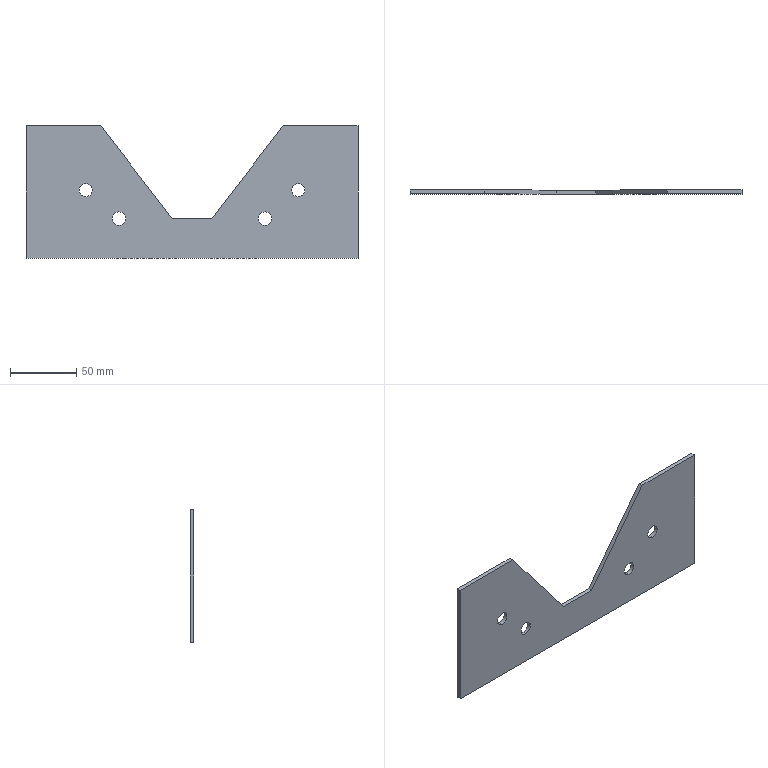Part | SolidWorks | features BaseBody 1 | 1 solid | 18 faces | box 250 x 3 x 100 mm | volume 56478 mm3 | plane 10 | cylinder 8 | commonest cylinder face diameters 10 x8
STEP:
#1=CARTESIAN_POINT('',(437.247,540.,-287.909));
#2=VERTEX_POINT('',#1);
#3=CARTESIAN_POINT('',(437.247,540.,-297.909));
#4=VERTEX_POINT('',#3);
#5=CARTESIAN_POINT('',(437.247,540.,-292.909));
#6=DIRECTION('',(0.,-1.,0.));
#7=DIRECTION('',(0.,0.,-1.));
#8=AXIS2_PLACEMENT_3D('',#5,#6,#7);
#9=CIRCLE('',#8,5.);
#10=EDGE_CURVE('',#2,#4,#9,.T.);
#11=ORIENTED_EDGE('',*,*,#10,.F.);
#12=CARTESIAN_POINT('',(437.247,537.,-287.909));
#13=VERTEX_POINT('',#12);
#14=CARTESIAN_POINT('',(437.247,547.,-287.909));
#15=DIRECTION('',(0.,-1.,0.));
#16=VECTOR('',#15,1000.);
#17=LINE('',#14,#16);
#18=EDGE_CURVE('',#2,#13,#17,.T.);
#19=ORIENTED_EDGE('',*,*,#18,.T.);
#20=CARTESIAN_POINT('',(437.247,537.,-297.909));
#21=VERTEX_POINT('',#20);
#22=CARTESIAN_POINT('',(437.247,537.,-292.909));
#23=DIRECTION('',(0.,1.,0.));
#24=DIRECTION('',(0.,0.,-1.));
#25=AXIS2_PLACEMENT_3D('',#22,#23,#24);
#26=CIRCLE('',#25,5.);
#27=EDGE_CURVE('',#21,#13,#26,.T.);
#28=ORIENTED_EDGE('',*,*,#27,.F.);
#29=CARTESIAN_POINT('',(437.247,547.,-297.909));
#30=DIRECTION('',(0.,-1.,0.));
#31=VECTOR('',#30,1000.);
#32=LINE('',#29,#31);
#33=EDGE_CURVE('',#4,#21,#32,.T.);
#34=ORIENTED_EDGE('',*,*,#33,.F.);
#35=EDGE_LOOP('',(#11,#19,#28,#34));
#36=FACE_OUTER_BOUND('',#35,.T.);
#37=CARTESIAN_POINT('',(437.247,547.,-292.909));
#38=DIRECTION('',(0.,-1.,0.));
#39=DIRECTION('',(0.,0.,-1.));
#40=AXIS2_PLACEMENT_3D('',#37,#38,#39);
#41=CYLINDRICAL_SURFACE('',#40,5.);
#42=ADVANCED_FACE('',(#36),#41,.F.);
#43=CARTESIAN_POINT('',(302.247,540.,-309.345));
#44=VERTEX_POINT('',#43);
#45=CARTESIAN_POINT('',(302.247,540.,-319.345));
#46=VERTEX_POINT('',#45);
#47=CARTESIAN_POINT('',(302.247,540.,-314.345));
#48=DIRECTION('',(0.,-1.,0.));
#49=DIRECTION('',(0.,0.,-1.));
#50=AXIS2_PLACEMENT_3D('',#47,#48,#49);
#51=CIRCLE('',#50,5.);
#52=EDGE_CURVE('',#44,#46,#51,.T.);
#53=ORIENTED_EDGE('',*,*,#52,.F.);
#54=CARTESIAN_POINT('',(302.247,537.,-309.345));
#55=VERTEX_POINT('',#54);
#56=CARTESIAN_POINT('',(302.247,547.,-309.345));
#57=DIRECTION('',(0.,-1.,0.));
#58=VECTOR('',#57,1000.);
#59=LINE('',#56,#58);
#60=EDGE_CURVE('',#44,#55,#59,.T.);
#61=ORIENTED_EDGE('',*,*,#60,.T.);
#62=CARTESIAN_POINT('',(302.247,537.,-319.345));
#63=VERTEX_POINT('',#62);
#64=CARTESIAN_POINT('',(302.247,537.,-314.345));
#65=DIRECTION('',(0.,1.,0.));
#66=DIRECTION('',(0.,0.,-1.));
#67=AXIS2_PLACEMENT_3D('',#64,#65,#66);
#68=CIRCLE('',#67,5.);
#69=EDGE_CURVE('',#63,#55,#68,.T.);
#70=ORIENTED_EDGE('',*,*,#69,.F.);
#71=CARTESIAN_POINT('',(302.247,547.,-319.345));
#72=DIRECTION('',(0.,-1.,0.));
#73=VECTOR('',#72,1000.);
#74=LINE('',#71,#73);
#75=EDGE_CURVE('',#46,#63,#74,.T.);
#76=ORIENTED_EDGE('',*,*,#75,.F.);
#77=EDGE_LOOP('',(#53,#61,#70,#76));
#78=FACE_OUTER_BOUND('',#77,.T.);
#79=CARTESIAN_POINT('',(302.247,547.,-314.345));
#80=DIRECTION('',(0.,-1.,0.));
#81=DIRECTION('',(0.,0.,-1.));
#82=AXIS2_PLACEMENT_3D('',#79,#80,#81);
#83=CYLINDRICAL_SURFACE('',#82,5.);
#84=ADVANCED_FACE('',(#78),#83,.F.);
#85=CARTESIAN_POINT('',(412.247,540.,-309.345));
#86=VERTEX_POINT('',#85);
#87=CARTESIAN_POINT('',(412.247,540.,-319.345));
#88=VERTEX_POINT('',#87);
#89=CARTESIAN_POINT('',(412.247,540.,-314.345));
#90=DIRECTION('',(0.,-1.,0.));
#91=DIRECTION('',(0.,0.,-1.));
#92=AXIS2_PLACEMENT_3D('',#89,#90,#91);
#93=CIRCLE('',#92,5.);
#94=EDGE_CURVE('',#86,#88,#93,.T.);
#95=ORIENTED_EDGE('',*,*,#94,.F.);
#96=CARTESIAN_POINT('',(412.247,537.,-309.345));
#97=VERTEX_POINT('',#96);
#98=CARTESIAN_POINT('',(412.247,547.,-309.345));
#99=DIRECTION('',(0.,-1.,0.));
#100=VECTOR('',#99,1000.);
#101=LINE('',#98,#100);
#102=EDGE_CURVE('',#86,#97,#101,.T.);
#103=ORIENTED_EDGE('',*,*,#102,.T.);
#104=CARTESIAN_POINT('',(412.247,537.,-319.345));
#105=VERTEX_POINT('',#104);
#106=CARTESIAN_POINT('',(412.247,537.,-314.345));
#107=DIRECTION('',(0.,1.,0.));
#108=DIRECTION('',(0.,0.,-1.));
#109=AXIS2_PLACEMENT_3D('',#106,#107,#108);
#110=CIRCLE('',#109,5.);
#111=EDGE_CURVE('',#105,#97,#110,.T.);
#112=ORIENTED_EDGE('',*,*,#111,.F.);
#113=CARTESIAN_POINT('',(412.247,547.,-319.345));
#114=DIRECTION('',(0.,-1.,0.));
#115=VECTOR('',#114,1000.);
#116=LINE('',#113,#115);
#117=EDGE_CURVE('',#88,#105,#116,.T.);
#118=ORIENTED_EDGE('',*,*,#117,.F.);
#119=EDGE_LOOP('',(#95,#103,#112,#118));
#120=FACE_OUTER_BOUND('',#119,.T.);
#121=CARTESIAN_POINT('',(412.247,547.,-314.345));
#122=DIRECTION('',(0.,-1.,0.));
#123=DIRECTION('',(0.,0.,-1.));
#124=AXIS2_PLACEMENT_3D('',#121,#122,#123);
#125=CYLINDRICAL_SURFACE('',#124,5.);
#126=ADVANCED_FACE('',(#120),#125,.F.);
#127=CARTESIAN_POINT('',(277.247,540.,-287.909));
#128=VERTEX_POINT('',#127);
#129=CARTESIAN_POINT('',(277.247,540.,-297.909));
#130=VERTEX_POINT('',#129);
#131=CARTESIAN_POINT('',(277.247,540.,-292.909));
#132=DIRECTION('',(0.,-1.,0.));
#133=DIRECTION('',(0.,0.,-1.));
#134=AXIS2_PLACEMENT_3D('',#131,#132,#133);
#135=CIRCLE('',#134,5.);
#136=EDGE_CURVE('',#128,#130,#135,.T.);
#137=ORIENTED_EDGE('',*,*,#136,.F.);
#138=CARTESIAN_POINT('',(277.247,537.,-287.909));
#139=VERTEX_POINT('',#138);
#140=CARTESIAN_POINT('',(277.247,547.,-287.909));
#141=DIRECTION('',(0.,-1.,0.));
#142=VECTOR('',#141,1000.);
#143=LINE('',#140,#142);
#144=EDGE_CURVE('',#128,#139,#143,.T.);
#145=ORIENTED_EDGE('',*,*,#144,.T.);
#146=CARTESIAN_POINT('',(277.247,537.,-297.909));
#147=VERTEX_POINT('',#146);
#148=CARTESIAN_POINT('',(277.247,537.,-292.909));
#149=DIRECTION('',(0.,1.,0.));
#150=DIRECTION('',(0.,0.,-1.));
#151=AXIS2_PLACEMENT_3D('',#148,#149,#150);
#152=CIRCLE('',#151,5.);
#153=EDGE_CURVE('',#147,#139,#152,.T.);
#154=ORIENTED_EDGE('',*,*,#153,.F.);
#155=CARTESIAN_POINT('',(277.247,547.,-297.909));
#156=DIRECTION('',(0.,-1.,0.));
#157=VECTOR('',#156,1000.);
#158=LINE('',#155,#157);
#159=EDGE_CURVE('',#130,#147,#158,.T.);
#160=ORIENTED_EDGE('',*,*,#159,.F.);
#161=EDGE_LOOP('',(#137,#145,#154,#160));
#162=FACE_OUTER_BOUND('',#161,.T.);
#163=CARTESIAN_POINT('',(277.247,547.,-292.909));
#164=DIRECTION('',(0.,-1.,0.));
#165=DIRECTION('',(0.,0.,-1.));
#166=AXIS2_PLACEMENT_3D('',#163,#164,#165);
#167=CYLINDRICAL_SURFACE('',#166,5.);
#168=ADVANCED_FACE('',(#162),#167,.F.);
#169=ORIENTED_EDGE('',*,*,#27,.T.);
#170=CARTESIAN_POINT('',(437.247,537.,-292.909));
#171=DIRECTION('',(0.,1.,0.));
#172=DIRECTION('',(0.,0.,-1.));
#173=AXIS2_PLACEMENT_3D('',#170,#171,#172);
#174=CIRCLE('',#173,5.);
#175=EDGE_CURVE('',#13,#21,#174,.T.);
#176=ORIENTED_EDGE('',*,*,#175,.T.);
#177=EDGE_LOOP('',(#169,#176));
#178=FACE_BOUND('',#177,.T.);
#179=ORIENTED_EDGE('',*,*,#69,.T.);
#180=CARTESIAN_POINT('',(302.247,537.,-314.345));
#181=DIRECTION('',(0.,1.,0.));
#182=DIRECTION('',(0.,0.,-1.));
#183=AXIS2_PLACEMENT_3D('',#180,#181,#182);
#184=CIRCLE('',#183,5.);
#185=EDGE_CURVE('',#55,#63,#184,.T.);
#186=ORIENTED_EDGE('',*,*,#185,.T.);
#187=EDGE_LOOP('',(#179,#186));
#188=FACE_BOUND('',#187,.T.);
#189=ORIENTED_EDGE('',*,*,#111,.T.);
#190=CARTESIAN_POINT('',(412.247,537.,-314.345));
#191=DIRECTION('',(0.,1.,0.));
#192=DIRECTION('',(0.,0.,-1.));
#193=AXIS2_PLACEMENT_3D('',#190,#191,#192);
#194=CIRCLE('',#193,5.);
#195=EDGE_CURVE('',#97,#105,#194,.T.);
#196=ORIENTED_EDGE('',*,*,#195,.T.);
#197=EDGE_LOOP('',(#189,#196));
#198=FACE_BOUND('',#197,.T.);
#199=ORIENTED_EDGE('',*,*,#153,.T.);
#200=CARTESIAN_POINT('',(277.247,537.,-292.909));
#201=DIRECTION('',(0.,1.,0.));
#202=DIRECTION('',(0.,0.,-1.));
#203=AXIS2_PLACEMENT_3D('',#200,#201,#202);
#204=CIRCLE('',#203,5.);
#205=EDGE_CURVE('',#139,#147,#204,.T.);
#206=ORIENTED_EDGE('',*,*,#205,.T.);
#207=EDGE_LOOP('',(#199,#206));
#208=FACE_BOUND('',#207,.T.);
#209=CARTESIAN_POINT('',(232.247,537.,-344.345));
#210=VERTEX_POINT('',#209);
#211=CARTESIAN_POINT('',(482.247,537.,-344.345));
#212=VERTEX_POINT('',#211);
#213=CARTESIAN_POINT('',(357.247,537.,-344.345));
#214=DIRECTION('',(1.,0.,0.));
#215=VECTOR('',#214,1000.);
#216=LINE('',#213,#215);
#217=EDGE_CURVE('',#210,#212,#216,.T.);
#218=ORIENTED_EDGE('',*,*,#217,.T.);
#219=CARTESIAN_POINT('',(482.247,537.,-244.345));
#220=VERTEX_POINT('',#219);
#221=CARTESIAN_POINT('',(482.247,537.,-344.345));
#222=DIRECTION('',(0.,0.,1.));
#223=VECTOR('',#222,1000.);
#224=LINE('',#221,#223);
#225=EDGE_CURVE('',#212,#220,#224,.T.);
#226=ORIENTED_EDGE('',*,*,#225,.T.);
#227=CARTESIAN_POINT('',(425.959,537.,-244.345));
#228=VERTEX_POINT('',#227);
#229=CARTESIAN_POINT('',(357.247,537.,-244.345));
#230=DIRECTION('',(-1.,0.,0.));
#231=VECTOR('',#230,1000.);
#232=LINE('',#229,#231);
#233=EDGE_CURVE('',#220,#228,#232,.T.);
#234=ORIENTED_EDGE('',*,*,#233,.T.);
#235=CARTESIAN_POINT('',(372.247,537.,-314.345));
#236=VERTEX_POINT('',#235);
#237=CARTESIAN_POINT('',(425.959,537.,-244.345));
#238=DIRECTION('',(-0.6088,0.,-0.7934));
#239=VECTOR('',#238,1000.);
#240=LINE('',#237,#239);
#241=EDGE_CURVE('',#228,#236,#240,.T.);
#242=ORIENTED_EDGE('',*,*,#241,.T.);
#243=CARTESIAN_POINT('',(342.247,537.,-314.345));
#244=VERTEX_POINT('',#243);
#245=CARTESIAN_POINT('',(357.247,537.,-314.345));
#246=DIRECTION('',(-1.,0.,0.));
#247=VECTOR('',#246,1000.);
#248=LINE('',#245,#247);
#249=EDGE_CURVE('',#236,#244,#248,.T.);
#250=ORIENTED_EDGE('',*,*,#249,.T.);
#251=CARTESIAN_POINT('',(288.534,537.,-244.345));
#252=VERTEX_POINT('',#251);
#253=CARTESIAN_POINT('',(342.247,537.,-314.345));
#254=DIRECTION('',(-0.6088,0.,0.7934));
#255=VECTOR('',#254,1000.);
#256=LINE('',#253,#255);
#257=EDGE_CURVE('',#244,#252,#256,.T.);
#258=ORIENTED_EDGE('',*,*,#257,.T.);
#259=CARTESIAN_POINT('',(232.247,537.,-244.345));
#260=VERTEX_POINT('',#259);
#261=CARTESIAN_POINT('',(357.247,537.,-244.345));
#262=DIRECTION('',(-1.,0.,0.));
#263=VECTOR('',#262,1000.);
#264=LINE('',#261,#263);
#265=EDGE_CURVE('',#252,#260,#264,.T.);
#266=ORIENTED_EDGE('',*,*,#265,.T.);
#267=CARTESIAN_POINT('',(232.247,537.,-344.345));
#268=DIRECTION('',(0.,0.,-1.));
#269=VECTOR('',#268,1000.);
#270=LINE('',#267,#269);
#271=EDGE_CURVE('',#260,#210,#270,.T.);
#272=ORIENTED_EDGE('',*,*,#271,.T.);
#273=EDGE_LOOP('',(#218,#226,#234,#242,#250,#258,#266,#272));
#274=FACE_OUTER_BOUND('',#273,.T.);
#275=CARTESIAN_POINT('',(357.247,537.,-344.345));
#276=DIRECTION('',(0.,-1.,0.));
#277=DIRECTION('',(0.,0.,-1.));
#278=AXIS2_PLACEMENT_3D('',#275,#276,#277);
#279=PLANE('',#278);
#280=ADVANCED_FACE('',(#178,#188,#198,#208,#274),#279,.T.);
#281=ORIENTED_EDGE('',*,*,#18,.F.);
#282=CARTESIAN_POINT('',(437.247,540.,-292.909));
#283=DIRECTION('',(0.,-1.,0.));
#284=DIRECTION('',(0.,0.,-1.));
#285=AXIS2_PLACEMENT_3D('',#282,#283,#284);
#286=CIRCLE('',#285,5.);
#287=EDGE_CURVE('',#4,#2,#286,.T.);
#288=ORIENTED_EDGE('',*,*,#287,.F.);
#289=ORIENTED_EDGE('',*,*,#33,.T.);
#290=ORIENTED_EDGE('',*,*,#175,.F.);
#291=EDGE_LOOP('',(#281,#288,#289,#290));
#292=FACE_OUTER_BOUND('',#291,.T.);
#293=CARTESIAN_POINT('',(437.247,547.,-292.909));
#294=DIRECTION('',(0.,-1.,0.));
#295=DIRECTION('',(0.,0.,-1.));
#296=AXIS2_PLACEMENT_3D('',#293,#294,#295);
#297=CYLINDRICAL_SURFACE('',#296,5.);
#298=ADVANCED_FACE('',(#292),#297,.F.);
#299=ORIENTED_EDGE('',*,*,#60,.F.);
#300=CARTESIAN_POINT('',(302.247,540.,-314.345));
#301=DIRECTION('',(0.,-1.,0.));
#302=DIRECTION('',(0.,0.,-1.));
#303=AXIS2_PLACEMENT_3D('',#300,#301,#302);
#304=CIRCLE('',#303,5.);
#305=EDGE_CURVE('',#46,#44,#304,.T.);
#306=ORIENTED_EDGE('',*,*,#305,.F.);
#307=ORIENTED_EDGE('',*,*,#75,.T.);
#308=ORIENTED_EDGE('',*,*,#185,.F.);
#309=EDGE_LOOP('',(#299,#306,#307,#308));
#310=FACE_OUTER_BOUND('',#309,.T.);
#311=CARTESIAN_POINT('',(302.247,547.,-314.345));
#312=DIRECTION('',(0.,-1.,0.));
#313=DIRECTION('',(0.,0.,-1.));
#314=AXIS2_PLACEMENT_3D('',#311,#312,#313);
#315=CYLINDRICAL_SURFACE('',#314,5.);
#316=ADVANCED_FACE('',(#310),#315,.F.);
#317=ORIENTED_EDGE('',*,*,#102,.F.);
#318=CARTESIAN_POINT('',(412.247,540.,-314.345));
#319=DIRECTION('',(0.,-1.,0.));
#320=DIRECTION('',(0.,0.,-1.));
#321=AXIS2_PLACEMENT_3D('',#318,#319,#320);
#322=CIRCLE('',#321,5.);
#323=EDGE_CURVE('',#88,#86,#322,.T.);
#324=ORIENTED_EDGE('',*,*,#323,.F.);
#325=ORIENTED_EDGE('',*,*,#117,.T.);
#326=ORIENTED_EDGE('',*,*,#195,.F.);
#327=EDGE_LOOP('',(#317,#324,#325,#326));
#328=FACE_OUTER_BOUND('',#327,.T.);
#329=CARTESIAN_POINT('',(412.247,547.,-314.345));
#330=DIRECTION('',(0.,-1.,0.));
#331=DIRECTION('',(0.,0.,-1.));
#332=AXIS2_PLACEMENT_3D('',#329,#330,#331);
#333=CYLINDRICAL_SURFACE('',#332,5.);
#334=ADVANCED_FACE('',(#328),#333,.F.);
#335=ORIENTED_EDGE('',*,*,#144,.F.);
#336=CARTESIAN_POINT('',(277.247,540.,-292.909));
#337=DIRECTION('',(0.,-1.,0.));
#338=DIRECTION('',(0.,0.,-1.));
#339=AXIS2_PLACEMENT_3D('',#336,#337,#338);
#340=CIRCLE('',#339,5.);
#341=EDGE_CURVE('',#130,#128,#340,.T.);
#342=ORIENTED_EDGE('',*,*,#341,.F.);
#343=ORIENTED_EDGE('',*,*,#159,.T.);
#344=ORIENTED_EDGE('',*,*,#205,.F.);
#345=EDGE_LOOP('',(#335,#342,#343,#344));
#346=FACE_OUTER_BOUND('',#345,.T.);
#347=CARTESIAN_POINT('',(277.247,547.,-292.909));
#348=DIRECTION('',(0.,-1.,0.));
#349=DIRECTION('',(0.,0.,-1.));
#350=AXIS2_PLACEMENT_3D('',#347,#348,#349);
#351=CYLINDRICAL_SURFACE('',#350,5.);
#352=ADVANCED_FACE('',(#346),#351,.F.);
#353=ORIENTED_EDGE('',*,*,#225,.F.);
#354=CARTESIAN_POINT('',(482.247,540.,-344.345));
#355=VERTEX_POINT('',#354);
#356=CARTESIAN_POINT('',(482.247,537.,-344.345));
#357=DIRECTION('',(0.,-1.,0.));
#358=VECTOR('',#357,1000.);
#359=LINE('',#356,#358);
#360=EDGE_CURVE('',#355,#212,#359,.T.);
#361=ORIENTED_EDGE('',*,*,#360,.F.);
#362=CARTESIAN_POINT('',(482.247,540.,-244.345));
#363=VERTEX_POINT('',#362);
#364=CARTESIAN_POINT('',(482.247,540.,-344.345));
#365=DIRECTION('',(0.,0.,-1.));
#366=VECTOR('',#365,1000.);
#367=LINE('',#364,#366);
#368=EDGE_CURVE('',#363,#355,#367,.T.);
#369=ORIENTED_EDGE('',*,*,#368,.F.);
#370=CARTESIAN_POINT('',(482.247,537.,-244.345));
#371=DIRECTION('',(0.,1.,0.));
#372=VECTOR('',#371,1000.);
#373=LINE('',#370,#372);
#374=EDGE_CURVE('',#220,#363,#373,.T.);
#375=ORIENTED_EDGE('',*,*,#374,.F.);
#376=EDGE_LOOP('',(#353,#361,#369,#375));
#377=FACE_OUTER_BOUND('',#376,.T.);
#378=CARTESIAN_POINT('',(482.247,537.,-344.345));
#379=DIRECTION('',(-1.,0.,0.));
#380=DIRECTION('',(0.,0.,1.));
#381=AXIS2_PLACEMENT_3D('',#378,#379,#380);
#382=PLANE('',#381);
#383=ADVANCED_FACE('',(#377),#382,.F.);
#384=ORIENTED_EDGE('',*,*,#217,.F.);
#385=CARTESIAN_POINT('',(232.247,540.,-344.345));
#386=VERTEX_POINT('',#385);
#387=CARTESIAN_POINT('',(232.247,537.,-344.345));
#388=DIRECTION('',(0.,-1.,0.));
#389=VECTOR('',#388,1000.);
#390=LINE('',#387,#389);
#391=EDGE_CURVE('',#386,#210,#390,.T.);
#392=ORIENTED_EDGE('',*,*,#391,.F.);
#393=CARTESIAN_POINT('',(232.247,540.,-344.345));
#394=DIRECTION('',(-1.,0.,0.));
#395=VECTOR('',#394,1000.);
#396=LINE('',#393,#395);
#397=EDGE_CURVE('',#355,#386,#396,.T.);
#398=ORIENTED_EDGE('',*,*,#397,.F.);
#399=ORIENTED_EDGE('',*,*,#360,.T.);
#400=EDGE_LOOP('',(#384,#392,#398,#399));
#401=FACE_OUTER_BOUND('',#400,.T.);
#402=CARTESIAN_POINT('',(232.247,537.,-344.345));
#403=DIRECTION('',(0.,0.,1.));
#404=DIRECTION('',(1.,0.,0.));
#405=AXIS2_PLACEMENT_3D('',#402,#403,#404);
#406=PLANE('',#405);
#407=ADVANCED_FACE('',(#401),#406,.F.);
#408=ORIENTED_EDGE('',*,*,#271,.F.);
#409=CARTESIAN_POINT('',(232.247,540.,-244.345));
#410=VERTEX_POINT('',#409);
#411=CARTESIAN_POINT('',(232.247,537.,-244.345));
#412=DIRECTION('',(0.,-1.,0.));
#413=VECTOR('',#412,1000.);
#414=LINE('',#411,#413);
#415=EDGE_CURVE('',#410,#260,#414,.T.);
#416=ORIENTED_EDGE('',*,*,#415,.F.);
#417=CARTESIAN_POINT('',(232.247,540.,-344.345));
#418=DIRECTION('',(0.,0.,1.));
#419=VECTOR('',#418,1000.);
#420=LINE('',#417,#419);
#421=EDGE_CURVE('',#386,#410,#420,.T.);
#422=ORIENTED_EDGE('',*,*,#421,.F.);
#423=ORIENTED_EDGE('',*,*,#391,.T.);
#424=EDGE_LOOP('',(#408,#416,#422,#423));
#425=FACE_OUTER_BOUND('',#424,.T.);
#426=CARTESIAN_POINT('',(232.247,537.,-344.345));
#427=DIRECTION('',(1.,0.,0.));
#428=DIRECTION('',(0.,0.,-1.));
#429=AXIS2_PLACEMENT_3D('',#426,#427,#428);
#430=PLANE('',#429);
#431=ADVANCED_FACE('',(#425),#430,.F.);
#432=ORIENTED_EDGE('',*,*,#265,.F.);
#433=CARTESIAN_POINT('',(288.534,540.,-244.345));
#434=VERTEX_POINT('',#433);
#435=CARTESIAN_POINT('',(288.534,537.,-244.345));
#436=DIRECTION('',(0.,-1.,0.));
#437=VECTOR('',#436,1000.);
#438=LINE('',#435,#437);
#439=EDGE_CURVE('',#434,#252,#438,.T.);
#440=ORIENTED_EDGE('',*,*,#439,.F.);
#441=CARTESIAN_POINT('',(232.247,540.,-244.345));
#442=DIRECTION('',(1.,0.,0.));
#443=VECTOR('',#442,1000.);
#444=LINE('',#441,#443);
#445=EDGE_CURVE('',#410,#434,#444,.T.);
#446=ORIENTED_EDGE('',*,*,#445,.F.);
#447=ORIENTED_EDGE('',*,*,#415,.T.);
#448=EDGE_LOOP('',(#432,#440,#446,#447));
#449=FACE_OUTER_BOUND('',#448,.T.);
#450=CARTESIAN_POINT('',(232.247,537.,-244.345));
#451=DIRECTION('',(0.,0.,-1.));
#452=DIRECTION('',(-1.,0.,0.));
#453=AXIS2_PLACEMENT_3D('',#450,#451,#452);
#454=PLANE('',#453);
#455=ADVANCED_FACE('',(#449),#454,.F.);
#456=ORIENTED_EDGE('',*,*,#257,.F.);
#457=CARTESIAN_POINT('',(342.247,540.,-314.345));
#458=VERTEX_POINT('',#457);
#459=CARTESIAN_POINT('',(342.247,537.,-314.345));
#460=DIRECTION('',(0.,-1.,0.));
#461=VECTOR('',#460,1000.);
#462=LINE('',#459,#461);
#463=EDGE_CURVE('',#458,#244,#462,.T.);
#464=ORIENTED_EDGE('',*,*,#463,.F.);
#465=CARTESIAN_POINT('',(288.534,540.,-244.345));
#466=DIRECTION('',(0.6088,0.,-0.7934));
#467=VECTOR('',#466,1000.);
#468=LINE('',#465,#467);
#469=EDGE_CURVE('',#434,#458,#468,.T.);
#470=ORIENTED_EDGE('',*,*,#469,.F.);
#471=ORIENTED_EDGE('',*,*,#439,.T.);
#472=EDGE_LOOP('',(#456,#464,#470,#471));
#473=FACE_OUTER_BOUND('',#472,.T.);
#474=CARTESIAN_POINT('',(288.534,537.,-244.345));
#475=DIRECTION('',(-0.7934,0.,-0.6088));
#476=DIRECTION('',(-0.6088,0.,0.7934));
#477=AXIS2_PLACEMENT_3D('',#474,#475,#476);
#478=PLANE('',#477);
#479=ADVANCED_FACE('',(#473),#478,.F.);
#480=ORIENTED_EDGE('',*,*,#249,.F.);
#481=CARTESIAN_POINT('',(372.247,540.,-314.345));
#482=VERTEX_POINT('',#481);
#483=CARTESIAN_POINT('',(372.247,537.,-314.345));
#484=DIRECTION('',(0.,-1.,0.));
#485=VECTOR('',#484,1000.);
#486=LINE('',#483,#485);
#487=EDGE_CURVE('',#482,#236,#486,.T.);
#488=ORIENTED_EDGE('',*,*,#487,.F.);
#489=CARTESIAN_POINT('',(342.247,540.,-314.345));
#490=DIRECTION('',(1.,0.,0.));
#491=VECTOR('',#490,1000.);
#492=LINE('',#489,#491);
#493=EDGE_CURVE('',#458,#482,#492,.T.);
#494=ORIENTED_EDGE('',*,*,#493,.F.);
#495=ORIENTED_EDGE('',*,*,#463,.T.);
#496=EDGE_LOOP('',(#480,#488,#494,#495));
#497=FACE_OUTER_BOUND('',#496,.T.);
#498=CARTESIAN_POINT('',(342.247,537.,-314.345));
#499=DIRECTION('',(0.,0.,-1.));
#500=DIRECTION('',(-1.,0.,0.));
#501=AXIS2_PLACEMENT_3D('',#498,#499,#500);
#502=PLANE('',#501);
#503=ADVANCED_FACE('',(#497),#502,.F.);
#504=ORIENTED_EDGE('',*,*,#241,.F.);
#505=CARTESIAN_POINT('',(425.959,540.,-244.345));
#506=VERTEX_POINT('',#505);
#507=CARTESIAN_POINT('',(425.959,537.,-244.345));
#508=DIRECTION('',(0.,-1.,0.));
#509=VECTOR('',#508,1000.);
#510=LINE('',#507,#509);
#511=EDGE_CURVE('',#506,#228,#510,.T.);
#512=ORIENTED_EDGE('',*,*,#511,.F.);
#513=CARTESIAN_POINT('',(425.959,540.,-244.345));
#514=DIRECTION('',(0.6088,0.,0.7934));
#515=VECTOR('',#514,1000.);
#516=LINE('',#513,#515);
#517=EDGE_CURVE('',#482,#506,#516,.T.);
#518=ORIENTED_EDGE('',*,*,#517,.F.);
#519=ORIENTED_EDGE('',*,*,#487,.T.);
#520=EDGE_LOOP('',(#504,#512,#518,#519));
#521=FACE_OUTER_BOUND('',#520,.T.);
#522=CARTESIAN_POINT('',(425.959,537.,-244.345));
#523=DIRECTION('',(0.7934,0.,-0.6088));
#524=DIRECTION('',(-0.6088,0.,-0.7934));
#525=AXIS2_PLACEMENT_3D('',#522,#523,#524);
#526=PLANE('',#525);
#527=ADVANCED_FACE('',(#521),#526,.F.);
#528=ORIENTED_EDGE('',*,*,#233,.F.);
#529=ORIENTED_EDGE('',*,*,#374,.T.);
#530=CARTESIAN_POINT('',(482.247,540.,-244.345));
#531=DIRECTION('',(1.,0.,0.));
#532=VECTOR('',#531,1000.);
#533=LINE('',#530,#532);
#534=EDGE_CURVE('',#506,#363,#533,.T.);
#535=ORIENTED_EDGE('',*,*,#534,.F.);
#536=ORIENTED_EDGE('',*,*,#511,.T.);
#537=EDGE_LOOP('',(#528,#529,#535,#536));
#538=FACE_OUTER_BOUND('',#537,.T.);
#539=CARTESIAN_POINT('',(482.247,537.,-244.345));
#540=DIRECTION('',(0.,0.,-1.));
#541=DIRECTION('',(-1.,0.,0.));
#542=AXIS2_PLACEMENT_3D('',#539,#540,#541);
#543=PLANE('',#542);
#544=ADVANCED_FACE('',(#538),#543,.F.);
#545=ORIENTED_EDGE('',*,*,#287,.T.);
#546=ORIENTED_EDGE('',*,*,#10,.T.);
#547=EDGE_LOOP('',(#545,#546));
#548=FACE_BOUND('',#547,.T.);
#549=ORIENTED_EDGE('',*,*,#305,.T.);
#550=ORIENTED_EDGE('',*,*,#52,.T.);
#551=EDGE_LOOP('',(#549,#550));
#552=FACE_BOUND('',#551,.T.);
#553=ORIENTED_EDGE('',*,*,#323,.T.);
#554=ORIENTED_EDGE('',*,*,#94,.T.);
#555=EDGE_LOOP('',(#553,#554));
#556=FACE_BOUND('',#555,.T.);
#557=ORIENTED_EDGE('',*,*,#341,.T.);
#558=ORIENTED_EDGE('',*,*,#136,.T.);
#559=EDGE_LOOP('',(#557,#558));
#560=FACE_BOUND('',#559,.T.);
#561=ORIENTED_EDGE('',*,*,#421,.T.);
#562=ORIENTED_EDGE('',*,*,#445,.T.);
#563=ORIENTED_EDGE('',*,*,#469,.T.);
#564=ORIENTED_EDGE('',*,*,#493,.T.);
#565=ORIENTED_EDGE('',*,*,#517,.T.);
#566=ORIENTED_EDGE('',*,*,#534,.T.);
#567=ORIENTED_EDGE('',*,*,#368,.T.);
#568=ORIENTED_EDGE('',*,*,#397,.T.);
#569=EDGE_LOOP('',(#561,#562,#563,#564,#565,#566,#567,#568));
#570=FACE_OUTER_BOUND('',#569,.T.);
#571=CARTESIAN_POINT('',(357.247,540.,-344.345));
#572=DIRECTION('',(0.,-1.,0.));
#573=DIRECTION('',(0.,0.,-1.));
#574=AXIS2_PLACEMENT_3D('',#571,#572,#573);
#575=PLANE('',#574);
#576=ADVANCED_FACE('',(#548,#552,#556,#560,#570),#575,.F.);
#577=CLOSED_SHELL('',(#42,#84,#126,#168,#280,#298,#316,#334,#352,#383,#407,#431,#455,#479,#503,#527,#544,#576));
#578=MANIFOLD_SOLID_BREP('',#577);
#579=CARTESIAN_POINT('',(0.,0.,0.));
#580=DIRECTION('',(0.,0.,1.));
#581=DIRECTION('',(1.,0.,0.));
#582=AXIS2_PLACEMENT_3D('',#579,#580,#581);
#583=(LENGTH_UNIT()NAMED_UNIT(*)SI_UNIT(.MILLI.,.METRE.));
#584=UNCERTAINTY_MEASURE_WITH_UNIT(LENGTH_MEASURE(0.00001),#583,'','');
#585=(NAMED_UNIT(*)PLANE_ANGLE_UNIT()SI_UNIT($,.RADIAN.));
#586=(NAMED_UNIT(*)SI_UNIT($,.STERADIAN.)SOLID_ANGLE_UNIT());
#587=(GEOMETRIC_REPRESENTATION_CONTEXT(3)GLOBAL_UNCERTAINTY_ASSIGNED_CONTEXT((#584))GLOBAL_UNIT_ASSIGNED_CONTEXT((#583,#585,#586))REPRESENTATION_CONTEXT('',''));
#588=ADVANCED_BREP_SHAPE_REPRESENTATION('',(#578,#582),#587);